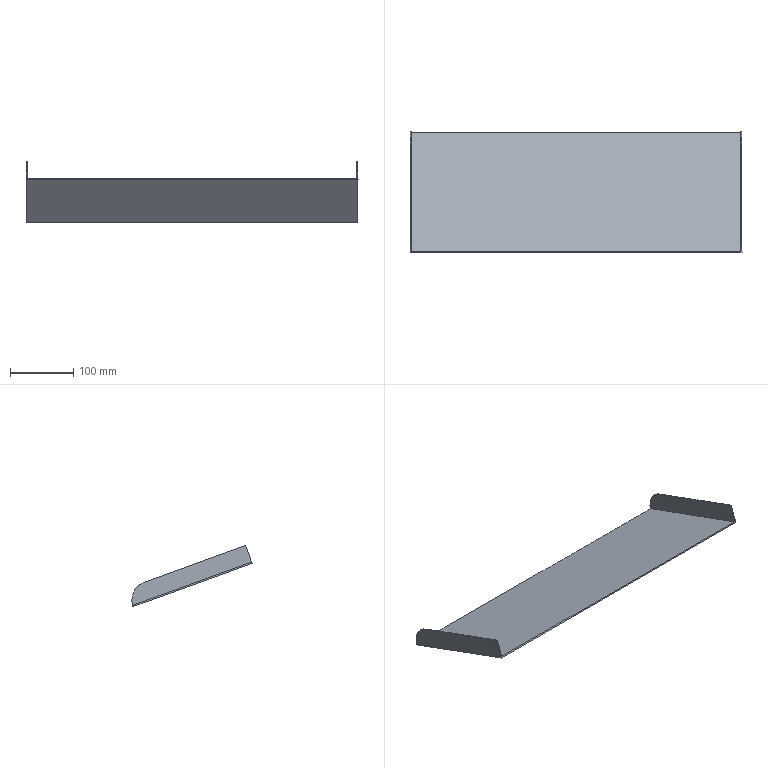Part | NX | features solid 2 | 1 solid | 12 faces | box 523.81 x 189.748 x 96.595 mm | volume 231152 mm3 | plane 10 | cylinder 2 | commonest cylinder face diameters 60 x2
STEP:
#1=CARTESIAN_POINT('',(-307.235,1009.316,-316.982));
#2=VERTEX_POINT('',#1);
#3=CARTESIAN_POINT('',(-831.045,1009.316,-316.982));
#4=VERTEX_POINT('',#3);
#5=CARTESIAN_POINT('',(-307.235,1009.316,-316.982));
#6=DIRECTION('',(1.,0.,0.));
#7=VECTOR('',#6,1000.);
#8=LINE('',#5,#7);
#9=EDGE_CURVE('',#2,#4,#8,.F.);
#10=ORIENTED_EDGE('',*,*,#9,.T.);
#11=CARTESIAN_POINT('',(-831.045,1197.254,-385.386));
#12=VERTEX_POINT('',#11);
#13=CARTESIAN_POINT('',(-831.045,1037.507,-327.243));
#14=DIRECTION('',(0.,0.9397,-0.342));
#15=VECTOR('',#14,1000.);
#16=LINE('',#13,#15);
#17=EDGE_CURVE('',#4,#12,#16,.T.);
#18=ORIENTED_EDGE('',*,*,#17,.T.);
#19=CARTESIAN_POINT('',(-307.235,1197.254,-385.386));
#20=VERTEX_POINT('',#19);
#21=CARTESIAN_POINT('',(-307.235,1197.254,-385.386));
#22=DIRECTION('',(1.,0.,0.));
#23=VECTOR('',#22,1000.);
#24=LINE('',#21,#23);
#25=EDGE_CURVE('',#20,#12,#24,.F.);
#26=ORIENTED_EDGE('',*,*,#25,.F.);
#27=CARTESIAN_POINT('',(-307.235,1009.316,-316.982));
#28=DIRECTION('',(0.,0.9397,-0.342));
#29=VECTOR('',#28,1000.);
#30=LINE('',#27,#29);
#31=EDGE_CURVE('',#2,#20,#30,.T.);
#32=ORIENTED_EDGE('',*,*,#31,.F.);
#33=EDGE_LOOP('',(#10,#18,#26,#32));
#34=FACE_BOUND('',#33,.T.);
#35=CARTESIAN_POINT('',(-307.235,1009.316,-316.982));
#36=DIRECTION('',(0.,-0.342,-0.9397));
#37=DIRECTION('',(0.,0.9397,-0.342));
#38=AXIS2_PLACEMENT_3D('',#35,#36,#37);
#39=PLANE('',#38);
#40=ADVANCED_FACE('',(#34),#39,.T.);
#41=CARTESIAN_POINT('',(-307.235,1019.577,-288.792));
#42=VERTEX_POINT('',#41);
#43=CARTESIAN_POINT('',(-307.235,1179.324,-346.935));
#44=VERTEX_POINT('',#43);
#45=CARTESIAN_POINT('',(-307.235,1019.577,-288.792));
#46=DIRECTION('',(0.,0.9397,-0.342));
#47=VECTOR('',#46,1000.);
#48=LINE('',#45,#47);
#49=EDGE_CURVE('',#42,#44,#48,.T.);
#50=ORIENTED_EDGE('',*,*,#49,.T.);
#51=CARTESIAN_POINT('',(-309.235,1179.324,-346.935));
#52=VERTEX_POINT('',#51);
#53=CARTESIAN_POINT('',(-307.235,1179.324,-346.935));
#54=DIRECTION('',(1.,0.,0.));
#55=VECTOR('',#54,1000.);
#56=LINE('',#53,#55);
#57=EDGE_CURVE('',#44,#52,#56,.F.);
#58=ORIENTED_EDGE('',*,*,#57,.T.);
#59=CARTESIAN_POINT('',(-309.235,1019.577,-288.792));
#60=VERTEX_POINT('',#59);
#61=CARTESIAN_POINT('',(-309.235,1019.577,-288.792));
#62=DIRECTION('',(0.,0.9397,-0.342));
#63=VECTOR('',#62,1000.);
#64=LINE('',#61,#63);
#65=EDGE_CURVE('',#60,#52,#64,.T.);
#66=ORIENTED_EDGE('',*,*,#65,.F.);
#67=CARTESIAN_POINT('',(-307.235,1019.577,-288.792));
#68=DIRECTION('',(1.,0.,0.));
#69=VECTOR('',#68,1000.);
#70=LINE('',#67,#69);
#71=EDGE_CURVE('',#42,#60,#70,.F.);
#72=ORIENTED_EDGE('',*,*,#71,.F.);
#73=EDGE_LOOP('',(#50,#58,#66,#72));
#74=FACE_BOUND('',#73,.T.);
#75=CARTESIAN_POINT('',(-307.235,1019.577,-288.792));
#76=DIRECTION('',(0.,-0.342,-0.9397));
#77=DIRECTION('',(0.,0.9397,-0.342));
#78=AXIS2_PLACEMENT_3D('',#75,#76,#77);
#79=PLANE('',#78);
#80=ADVANCED_FACE('',(#74),#79,.F.);
#81=CARTESIAN_POINT('',(-829.045,1010.,-315.103));
#82=VERTEX_POINT('',#81);
#83=CARTESIAN_POINT('',(-309.235,1010.,-315.103));
#84=VERTEX_POINT('',#83);
#85=CARTESIAN_POINT('',(-819.045,1010.,-315.103));
#86=DIRECTION('',(-1.,0.,0.));
#87=VECTOR('',#86,1000.);
#88=LINE('',#85,#87);
#89=EDGE_CURVE('',#82,#84,#88,.F.);
#90=ORIENTED_EDGE('',*,*,#89,.F.);
#91=CARTESIAN_POINT('',(-829.045,1019.577,-288.792));
#92=VERTEX_POINT('',#91);
#93=CARTESIAN_POINT('',(-829.045,1009.316,-316.982));
#94=DIRECTION('',(0.,-0.342,-0.9397));
#95=VECTOR('',#94,1000.);
#96=LINE('',#93,#95);
#97=EDGE_CURVE('',#82,#92,#96,.F.);
#98=ORIENTED_EDGE('',*,*,#97,.T.);
#99=CARTESIAN_POINT('',(-831.045,1019.577,-288.792));
#100=VERTEX_POINT('',#99);
#101=CARTESIAN_POINT('',(-831.045,1019.577,-288.792));
#102=DIRECTION('',(1.,0.,0.));
#103=VECTOR('',#102,1000.);
#104=LINE('',#101,#103);
#105=EDGE_CURVE('',#100,#92,#104,.T.);
#106=ORIENTED_EDGE('',*,*,#105,.F.);
#107=CARTESIAN_POINT('',(-831.045,1010.,-315.103));
#108=DIRECTION('',(0.,0.342,0.9397));
#109=VECTOR('',#108,1000.);
#110=LINE('',#107,#109);
#111=EDGE_CURVE('',#100,#4,#110,.F.);
#112=ORIENTED_EDGE('',*,*,#111,.T.);
#113=ORIENTED_EDGE('',*,*,#9,.F.);
#114=CARTESIAN_POINT('',(-307.235,1009.316,-316.982));
#115=DIRECTION('',(0.,0.342,0.9397));
#116=VECTOR('',#115,1000.);
#117=LINE('',#114,#116);
#118=EDGE_CURVE('',#2,#42,#117,.T.);
#119=ORIENTED_EDGE('',*,*,#118,.T.);
#120=ORIENTED_EDGE('',*,*,#71,.T.);
#121=CARTESIAN_POINT('',(-309.235,1009.316,-316.982));
#122=DIRECTION('',(0.,-0.342,-0.9397));
#123=VECTOR('',#122,1000.);
#124=LINE('',#121,#123);
#125=EDGE_CURVE('',#84,#60,#124,.F.);
#126=ORIENTED_EDGE('',*,*,#125,.F.);
#127=EDGE_LOOP('',(#90,#98,#106,#112,#113,#119,#120,#126));
#128=FACE_BOUND('',#127,.T.);
#129=CARTESIAN_POINT('',(-307.235,1009.316,-316.982));
#130=DIRECTION('',(0.,0.9397,-0.342));
#131=DIRECTION('',(0.,0.342,0.9397));
#132=AXIS2_PLACEMENT_3D('',#129,#130,#131);
#133=PLANE('',#132);
#134=ADVANCED_FACE('',(#128),#133,.F.);
#135=CARTESIAN_POINT('',(-309.235,1197.876,-383.484));
#136=VERTEX_POINT('',#135);
#137=CARTESIAN_POINT('',(-309.235,1169.064,-375.126));
#138=DIRECTION('',(1.,0.,0.));
#139=DIRECTION('',(0.,-0.342,-0.9397));
#140=AXIS2_PLACEMENT_3D('',#137,#138,#139);
#141=CIRCLE('',#140,30.);
#142=EDGE_CURVE('',#52,#136,#141,.F.);
#143=ORIENTED_EDGE('',*,*,#142,.T.);
#144=CARTESIAN_POINT('',(-309.235,1010.,-315.103));
#145=DIRECTION('',(0.,-0.9397,0.342));
#146=VECTOR('',#145,1000.);
#147=LINE('',#144,#146);
#148=EDGE_CURVE('',#136,#84,#147,.T.);
#149=ORIENTED_EDGE('',*,*,#148,.T.);
#150=ORIENTED_EDGE('',*,*,#125,.T.);
#151=ORIENTED_EDGE('',*,*,#65,.T.);
#152=EDGE_LOOP('',(#143,#149,#150,#151));
#153=FACE_BOUND('',#152,.T.);
#154=CARTESIAN_POINT('',(-309.235,1009.316,-316.982));
#155=DIRECTION('',(1.,0.,0.));
#156=DIRECTION('',(0.,-0.342,-0.9397));
#157=AXIS2_PLACEMENT_3D('',#154,#155,#156);
#158=PLANE('',#157);
#159=ADVANCED_FACE('',(#153),#158,.F.);
#160=ORIENTED_EDGE('',*,*,#49,.F.);
#161=ORIENTED_EDGE('',*,*,#118,.F.);
#162=ORIENTED_EDGE('',*,*,#31,.T.);
#163=CARTESIAN_POINT('',(-307.235,1197.939,-383.507));
#164=VERTEX_POINT('',#163);
#165=CARTESIAN_POINT('',(-307.235,1197.939,-383.507));
#166=DIRECTION('',(0.,0.342,0.9397));
#167=VECTOR('',#166,1000.);
#168=LINE('',#165,#167);
#169=EDGE_CURVE('',#164,#20,#168,.F.);
#170=ORIENTED_EDGE('',*,*,#169,.F.);
#171=CARTESIAN_POINT('',(-307.235,1197.876,-383.484));
#172=VERTEX_POINT('',#171);
#173=CARTESIAN_POINT('',(-307.235,1038.191,-325.364));
#174=DIRECTION('',(0.,-0.9397,0.342));
#175=VECTOR('',#174,1000.);
#176=LINE('',#173,#175);
#177=EDGE_CURVE('',#172,#164,#176,.F.);
#178=ORIENTED_EDGE('',*,*,#177,.F.);
#179=CARTESIAN_POINT('',(-307.235,1169.064,-375.126));
#180=DIRECTION('',(1.,0.,0.));
#181=DIRECTION('',(0.,-0.342,-0.9397));
#182=AXIS2_PLACEMENT_3D('',#179,#180,#181);
#183=CIRCLE('',#182,30.);
#184=EDGE_CURVE('',#172,#44,#183,.T.);
#185=ORIENTED_EDGE('',*,*,#184,.T.);
#186=EDGE_LOOP('',(#160,#161,#162,#170,#178,#185));
#187=FACE_BOUND('',#186,.T.);
#188=CARTESIAN_POINT('',(-307.235,1009.316,-316.982));
#189=DIRECTION('',(1.,0.,0.));
#190=DIRECTION('',(0.,-0.342,-0.9397));
#191=AXIS2_PLACEMENT_3D('',#188,#189,#190);
#192=PLANE('',#191);
#193=ADVANCED_FACE('',(#187),#192,.T.);
#194=CARTESIAN_POINT('',(-309.235,1197.876,-383.484));
#195=CARTESIAN_POINT('',(-308.568,1197.876,-383.484));
#196=CARTESIAN_POINT('',(-307.902,1197.876,-383.484));
#197=CARTESIAN_POINT('',(-307.235,1197.876,-383.484));
#198=B_SPLINE_CURVE_WITH_KNOTS('',3,(#194,#195,#196,#197),.UNSPECIFIED.,.F.,.F.,(4,4),(1310.699,1310.701),.UNSPECIFIED.);
#199=EDGE_CURVE('',#136,#172,#198,.T.);
#200=ORIENTED_EDGE('',*,*,#199,.F.);
#201=ORIENTED_EDGE('',*,*,#142,.F.);
#202=ORIENTED_EDGE('',*,*,#57,.F.);
#203=ORIENTED_EDGE('',*,*,#184,.F.);
#204=EDGE_LOOP('',(#200,#201,#202,#203));
#205=FACE_BOUND('',#204,.T.);
#206=CARTESIAN_POINT('',(-307.235,1169.064,-375.126));
#207=DIRECTION('',(1.,0.,0.));
#208=DIRECTION('',(0.,-0.342,-0.9397));
#209=AXIS2_PLACEMENT_3D('',#206,#207,#208);
#210=CYLINDRICAL_SURFACE('',#209,30.);
#211=ADVANCED_FACE('',(#205),#210,.T.);
#212=CARTESIAN_POINT('',(-829.045,1197.876,-383.484));
#213=VERTEX_POINT('',#212);
#214=CARTESIAN_POINT('',(-829.045,1038.191,-325.364));
#215=DIRECTION('',(0.,0.9397,-0.342));
#216=VECTOR('',#215,1000.);
#217=LINE('',#214,#216);
#218=EDGE_CURVE('',#82,#213,#217,.T.);
#219=ORIENTED_EDGE('',*,*,#218,.F.);
#220=ORIENTED_EDGE('',*,*,#89,.T.);
#221=ORIENTED_EDGE('',*,*,#148,.F.);
#222=ORIENTED_EDGE('',*,*,#199,.T.);
#223=ORIENTED_EDGE('',*,*,#177,.T.);
#224=CARTESIAN_POINT('',(-831.045,1197.939,-383.507));
#225=VERTEX_POINT('',#224);
#226=CARTESIAN_POINT('',(-819.045,1197.939,-383.507));
#227=DIRECTION('',(1.,0.,0.));
#228=VECTOR('',#227,1000.);
#229=LINE('',#226,#228);
#230=EDGE_CURVE('',#225,#164,#229,.T.);
#231=ORIENTED_EDGE('',*,*,#230,.F.);
#232=CARTESIAN_POINT('',(-831.045,1197.876,-383.484));
#233=VERTEX_POINT('',#232);
#234=CARTESIAN_POINT('',(-831.045,1038.191,-325.364));
#235=DIRECTION('',(0.,0.9397,-0.342));
#236=VECTOR('',#235,1000.);
#237=LINE('',#234,#236);
#238=EDGE_CURVE('',#233,#225,#237,.T.);
#239=ORIENTED_EDGE('',*,*,#238,.F.);
#240=CARTESIAN_POINT('',(-829.045,1197.876,-383.484));
#241=CARTESIAN_POINT('',(-829.712,1197.876,-383.484));
#242=CARTESIAN_POINT('',(-830.378,1197.876,-383.484));
#243=CARTESIAN_POINT('',(-831.045,1197.876,-383.484));
#244=B_SPLINE_CURVE_WITH_KNOTS('',3,(#240,#241,#242,#243),.UNSPECIFIED.,.F.,.F.,(4,4),(1310.699,1310.701),.UNSPECIFIED.);
#245=EDGE_CURVE('',#213,#233,#244,.T.);
#246=ORIENTED_EDGE('',*,*,#245,.F.);
#247=EDGE_LOOP('',(#219,#220,#221,#222,#223,#231,#239,#246));
#248=FACE_BOUND('',#247,.T.);
#249=CARTESIAN_POINT('',(-819.045,1038.191,-325.364));
#250=DIRECTION('',(0.,0.342,0.9397));
#251=DIRECTION('',(1.,0.,0.));
#252=AXIS2_PLACEMENT_3D('',#249,#250,#251);
#253=PLANE('',#252);
#254=ADVANCED_FACE('',(#248),#253,.T.);
#255=ORIENTED_EDGE('',*,*,#169,.T.);
#256=ORIENTED_EDGE('',*,*,#25,.T.);
#257=CARTESIAN_POINT('',(-831.045,1197.939,-383.507));
#258=DIRECTION('',(0.,-0.342,-0.9397));
#259=VECTOR('',#258,1000.);
#260=LINE('',#257,#259);
#261=EDGE_CURVE('',#225,#12,#260,.T.);
#262=ORIENTED_EDGE('',*,*,#261,.F.);
#263=ORIENTED_EDGE('',*,*,#230,.T.);
#264=EDGE_LOOP('',(#255,#256,#262,#263));
#265=FACE_BOUND('',#264,.T.);
#266=CARTESIAN_POINT('',(-819.045,1197.939,-383.507));
#267=DIRECTION('',(0.,-0.9397,0.342));
#268=DIRECTION('',(1.,0.,0.));
#269=AXIS2_PLACEMENT_3D('',#266,#267,#268);
#270=PLANE('',#269);
#271=ADVANCED_FACE('',(#265),#270,.F.);
#272=ORIENTED_EDGE('',*,*,#261,.T.);
#273=ORIENTED_EDGE('',*,*,#17,.F.);
#274=ORIENTED_EDGE('',*,*,#111,.F.);
#275=CARTESIAN_POINT('',(-831.045,1179.324,-346.935));
#276=VERTEX_POINT('',#275);
#277=CARTESIAN_POINT('',(-831.045,1019.577,-288.792));
#278=DIRECTION('',(0.,0.9397,-0.342));
#279=VECTOR('',#278,1000.);
#280=LINE('',#277,#279);
#281=EDGE_CURVE('',#100,#276,#280,.T.);
#282=ORIENTED_EDGE('',*,*,#281,.T.);
#283=CARTESIAN_POINT('',(-831.045,1169.064,-375.126));
#284=DIRECTION('',(1.,0.,0.));
#285=DIRECTION('',(0.,-0.342,-0.9397));
#286=AXIS2_PLACEMENT_3D('',#283,#284,#285);
#287=CIRCLE('',#286,30.);
#288=EDGE_CURVE('',#276,#233,#287,.F.);
#289=ORIENTED_EDGE('',*,*,#288,.T.);
#290=ORIENTED_EDGE('',*,*,#238,.T.);
#291=EDGE_LOOP('',(#272,#273,#274,#282,#289,#290));
#292=FACE_BOUND('',#291,.T.);
#293=CARTESIAN_POINT('',(-831.045,1038.191,-325.364));
#294=DIRECTION('',(1.,0.,0.));
#295=DIRECTION('',(0.,0.9397,-0.342));
#296=AXIS2_PLACEMENT_3D('',#293,#294,#295);
#297=PLANE('',#296);
#298=ADVANCED_FACE('',(#292),#297,.F.);
#299=CARTESIAN_POINT('',(-829.045,1179.324,-346.935));
#300=VERTEX_POINT('',#299);
#301=CARTESIAN_POINT('',(-829.045,1019.577,-288.792));
#302=DIRECTION('',(0.,0.9397,-0.342));
#303=VECTOR('',#302,1000.);
#304=LINE('',#301,#303);
#305=EDGE_CURVE('',#92,#300,#304,.T.);
#306=ORIENTED_EDGE('',*,*,#305,.T.);
#307=CARTESIAN_POINT('',(-831.045,1179.324,-346.935));
#308=DIRECTION('',(1.,0.,0.));
#309=VECTOR('',#308,1000.);
#310=LINE('',#307,#309);
#311=EDGE_CURVE('',#300,#276,#310,.F.);
#312=ORIENTED_EDGE('',*,*,#311,.T.);
#313=ORIENTED_EDGE('',*,*,#281,.F.);
#314=ORIENTED_EDGE('',*,*,#105,.T.);
#315=EDGE_LOOP('',(#306,#312,#313,#314));
#316=FACE_BOUND('',#315,.T.);
#317=CARTESIAN_POINT('',(-831.045,1019.577,-288.792));
#318=DIRECTION('',(0.,-0.342,-0.9397));
#319=DIRECTION('',(0.,0.9397,-0.342));
#320=AXIS2_PLACEMENT_3D('',#317,#318,#319);
#321=PLANE('',#320);
#322=ADVANCED_FACE('',(#316),#321,.F.);
#323=ORIENTED_EDGE('',*,*,#97,.F.);
#324=ORIENTED_EDGE('',*,*,#218,.T.);
#325=CARTESIAN_POINT('',(-829.045,1169.064,-375.126));
#326=DIRECTION('',(1.,0.,0.));
#327=DIRECTION('',(0.,-0.342,-0.9397));
#328=AXIS2_PLACEMENT_3D('',#325,#326,#327);
#329=CIRCLE('',#328,30.);
#330=EDGE_CURVE('',#213,#300,#329,.T.);
#331=ORIENTED_EDGE('',*,*,#330,.T.);
#332=ORIENTED_EDGE('',*,*,#305,.F.);
#333=EDGE_LOOP('',(#323,#324,#331,#332));
#334=FACE_BOUND('',#333,.T.);
#335=CARTESIAN_POINT('',(-829.045,1009.316,-316.982));
#336=DIRECTION('',(1.,0.,0.));
#337=DIRECTION('',(0.,-0.342,-0.9397));
#338=AXIS2_PLACEMENT_3D('',#335,#336,#337);
#339=PLANE('',#338);
#340=ADVANCED_FACE('',(#334),#339,.T.);
#341=ORIENTED_EDGE('',*,*,#330,.F.);
#342=ORIENTED_EDGE('',*,*,#245,.T.);
#343=ORIENTED_EDGE('',*,*,#288,.F.);
#344=ORIENTED_EDGE('',*,*,#311,.F.);
#345=EDGE_LOOP('',(#341,#342,#343,#344));
#346=FACE_BOUND('',#345,.T.);
#347=CARTESIAN_POINT('',(-831.045,1169.064,-375.126));
#348=DIRECTION('',(-1.,0.,0.));
#349=DIRECTION('',(0.,0.342,0.9397));
#350=AXIS2_PLACEMENT_3D('',#347,#348,#349);
#351=CYLINDRICAL_SURFACE('',#350,30.);
#352=ADVANCED_FACE('',(#346),#351,.T.);
#353=CLOSED_SHELL('',(#40,#80,#134,#159,#193,#211,#254,#271,#298,#322,#340,#352));
#354=MANIFOLD_SOLID_BREP('',#353);
#355=(LENGTH_UNIT()NAMED_UNIT(*)SI_UNIT(.MILLI.,.METRE.));
#356=UNCERTAINTY_MEASURE_WITH_UNIT(LENGTH_MEASURE(0.0508),#355,'','');
#357=(NAMED_UNIT(*)PLANE_ANGLE_UNIT()SI_UNIT($,.RADIAN.));
#358=(NAMED_UNIT(*)SI_UNIT($,.STERADIAN.)SOLID_ANGLE_UNIT());
#359=(GEOMETRIC_REPRESENTATION_CONTEXT(3)GLOBAL_UNCERTAINTY_ASSIGNED_CONTEXT((#356))GLOBAL_UNIT_ASSIGNED_CONTEXT((#355,#357,#358))REPRESENTATION_CONTEXT('',''));
#360=ADVANCED_BREP_SHAPE_REPRESENTATION('',(#354),#359);